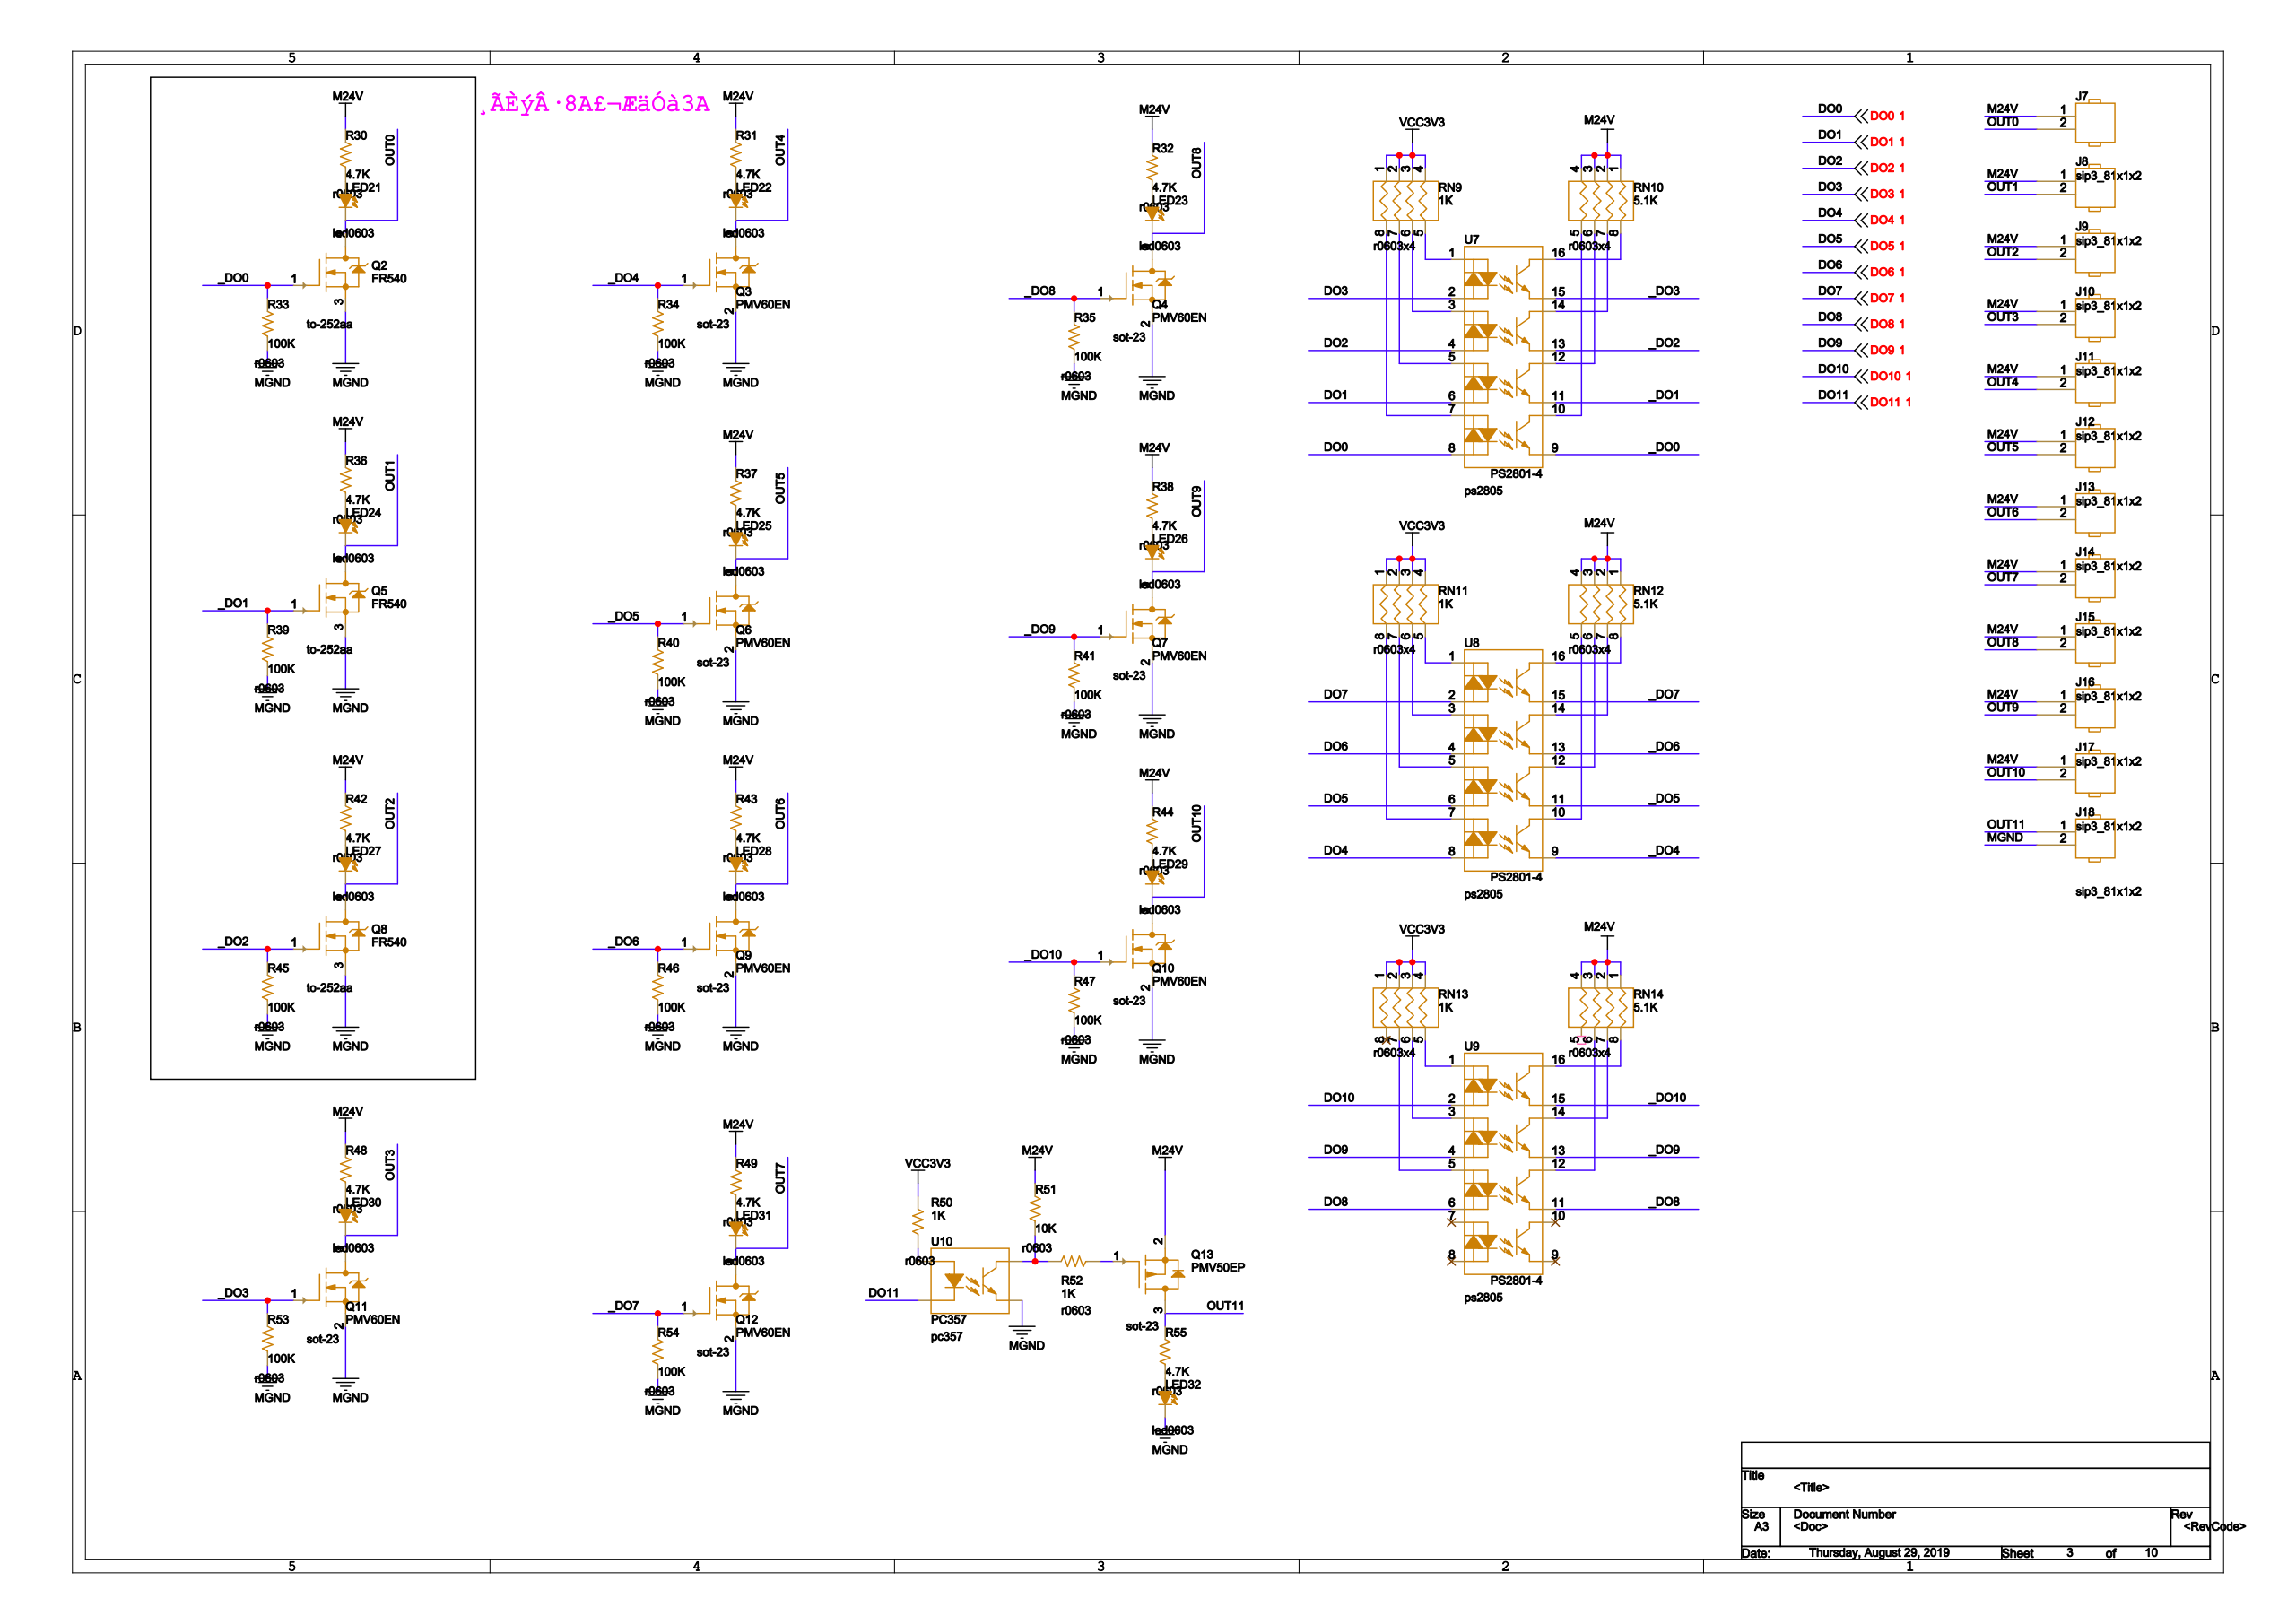Circuit board | Cadence Allegro | 380 parts | 375 nets | one sheet of the schematic
Parts on this sheet (reference | value | footprint):
J7 | HEADER 2 | SIP3_81X1X2
J8 | HEADER 2 | SIP3_81X1X2
J9 | HEADER 2 | SIP3_81X1X2
J10 | HEADER 2 | SIP3_81X1X2
J11 | HEADER 2 | SIP3_81X1X2
J12 | HEADER 2 | SIP3_81X1X2
J13 | HEADER 2 | SIP3_81X1X2
J14 | HEADER 2 | SIP3_81X1X2
J15 | HEADER 2 | SIP3_81X1X2
J16 | HEADER 2 | SIP3_81X1X2
J17 | HEADER 2 | SIP3_81X1X2
J18 | HEADER 2 | SIP3_81X1X2
LED21 | LED | LED0603
LED22 | LED | LED0603
LED23 | LED | LED0603
LED24 | LED | LED0603
LED25 | LED | LED0603
LED26 | LED | LED0603
LED27 | LED | LED0603
LED28 | LED | LED0603
LED29 | LED | LED0603
LED30 | LED | LED0603
LED31 | LED | LED0603
LED32 | LED | LED0603
Q2 | FR540 | TO-252AA
Q3 | PMV60EN | SOT-23
Q4 | PMV60EN | SOT-23
Q5 | FR540 | TO-252AA
Q6 | PMV60EN | SOT-23
Q7 | PMV60EN | SOT-23
Q8 | FR540 | TO-252AA
Q9 | PMV60EN | SOT-23
Q10 | PMV60EN | SOT-23
Q11 | PMV60EN | SOT-23
Q12 | PMV60EN | SOT-23
Q13 | PMV50EP | SOT-23
R30 | 4.7K | R0603
R31 | 4.7K | R0603
R32 | 4.7K | R0603
R33 | 100K | R0603
R34 | 100K | R0603
R35 | 100K | R0603
R36 | 4.7K | R0603
R37 | 4.7K | R0603
R38 | 4.7K | R0603
R39 | 100K | R0603
R40 | 100K | R0603
R41 | 100K | R0603
R42 | 4.7K | R0603
R43 | 4.7K | R0603
R44 | 4.7K | R0603
R45 | 100K | R0603
R46 | 100K | R0603
R47 | 100K | R0603
R48 | 4.7K | R0603
R49 | 4.7K | R0603
R50 | 1K | R0603
R51 | 10K | R0603
R52 | 1K | R0603
R53 | 100K | R0603
R54 | 100K | R0603
R55 | 4.7K | R0603
RN9 | 1K | R0603X4
RN10 | 5.1K | R0603X4
RN11 | 1K | R0603X4
RN12 | 5.1K | R0603X4
RN13 | 1K | R0603X4
RN14 | 5.1K | R0603X4
U7 | PS2801-4 | PS2805
U8 | PS2801-4 | PS2805
U9 | PS2801-4 | PS2805
U10 | PC357 | PC357
Nets of these parts (net: part-pin ...):
M24V: J7-1 J8-1 J9-1 J10-1 J11-1 J12-1 J13-1 J14-1 J15-1 J16-1 J17-1 Q13-2 R30-2 R31-2 R32-2 R36-2 R37-2 R38-2 R42-2 R43-2 R44-2 R48-2 R49-2 R51-2 RN10-1 RN10-2 RN10-3 RN10-4 RN12-1 RN12-2 RN12-3 RN12-4 RN14-1 RN14-2 RN14-3 RN14-4
N1825115: RN10-5 U7-10
N1825123: RN10-6 U7-12
N1825131: RN10-7 U7-14
N1825139: RN10-8 U7-16
N1825923: RN12-5 U8-10
N1825947: RN12-6 U8-12
N1825939: RN12-7 U8-14
N1825961: RN12-8 U8-16
N1826388: RN14-6 U9-12
N1826380: RN14-7 U9-14
N1826402: RN14-8 U9-16
VCC3V3: R50-2 RN9-1 RN9-2 RN9-3 RN9-4 RN11-1 RN11-2 RN11-3 RN11-4 RN13-1 RN13-2 RN13-3 RN13-4
N1826197: RN11-5 U8-1
N1826213: RN11-6 U8-3
N1826205: RN11-7 U8-5
N1825931: RN11-8 U8-7
N1826638: RN13-5 U9-1
N1826654: RN13-6 U9-3
N1826646: RN13-7 U9-5
N1825083: RN9-5 U7-1
N1825091: RN9-6 U7-3
N1825099: RN9-7 U7-5
N1825107: RN9-8 U7-7
_DO1: Q5-1 R39-2 U7-11
_DO2: Q8-1 R45-2 U7-13
_DO3: Q11-1 R53-2 U7-15
DO3: U7-2
DO2: U7-4
DO1: U7-6
DO0: U7-8
_DO0: Q2-1 R33-2 U7-9
_DO5: Q6-1 R40-2 U8-11
_DO6: Q9-1 R46-2 U8-13
_DO7: Q12-1 R54-2 U8-15
DO7: U8-2
DO6: U8-4
DO5: U8-6
DO4: U8-8
_DO4: Q3-1 R34-2 U8-9
_DO8: Q4-1 R35-2 U9-11
_DO9: Q7-1 R41-2 U9-13
_DO10: Q10-1 R47-2 U9-15
DO10: U9-2
DO9: U9-4
DO8: U9-6
OUT11: J18-1 Q13-3 R55-2
N1733182: Q13-1 R52-1
MGND: J18-2 LED32-2 Q2-3 Q3-2 Q4-2 Q5-3 Q6-2 Q7-2 Q8-3 Q9-2 Q10-2 Q11-2 Q12-2 R33-1 R34-1 R35-1 R39-1 R40-1 R41-1 R45-1 R46-1 R47-1 R53-1 R54-1 U10-3
OUT3: J10-2 LED30-2 Q11-3
OUT4: J11-2 LED22-2 Q3-3
OUT5: J12-2 LED25-2 Q6-3
OUT6: J13-2 LED28-2 Q9-3
OUT7: J14-2 LED31-2 Q12-3
OUT8: J15-2 LED23-2 Q4-3
OUT9: J16-2 LED26-2 Q7-3
OUT10: J17-2 LED29-2 Q10-3
OUT0: J7-2 LED21-2 Q2-4
OUT1: J8-2 LED24-2 Q5-4
OUT2: J9-2 LED27-2 Q8-4
N15703391: LED21-1 R30-1
N15788751: LED22-1 R31-1
N15804171: LED23-1 R32-1
N15780771: LED24-1 R36-1
N15791341: LED25-1 R37-1
N15806311: LED26-1 R38-1
N15783171: LED27-1 R42-1
N15794461: LED28-1 R43-1
N15800371: LED29-1 R44-1
N15785621: LED30-1 R48-1
N15797231: LED31-1 R49-1
N17331061: LED32-1 R55-1
N1733186: R51-1 R52-2 U10-4
N1733094: R50-1 U10-1
DO11: U10-2